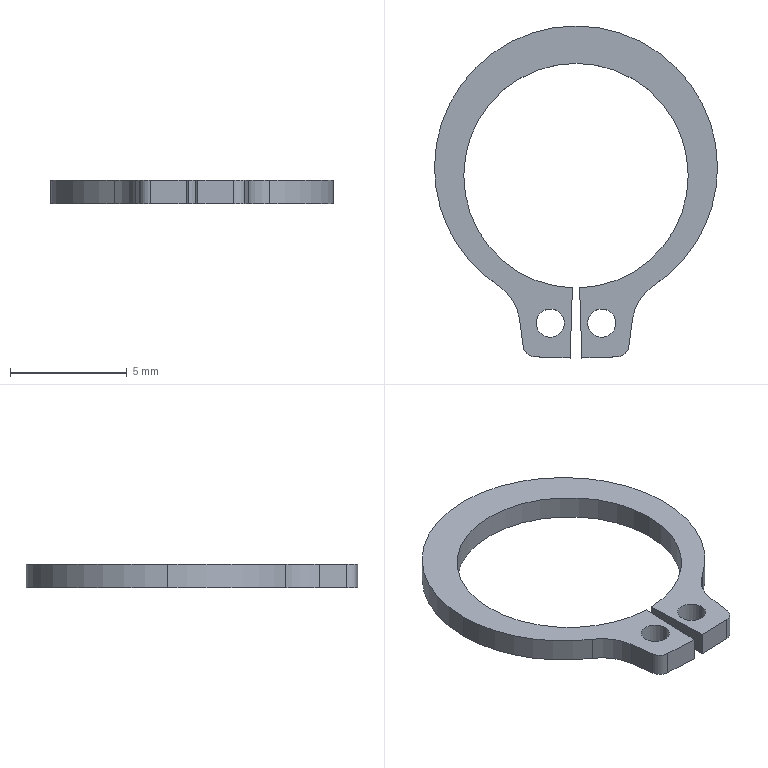Part | STEP file | C Type Shaft Use Retaining Ring_jis(PreviewCfg) | 1 solid | 22 faces | box 12.101 x 14.196 x 1 mm | volume 49.912 mm3 | cylinder 14 | plane 8 | commonest cylinder face diameters 1.2 x4 9.6 x3 12.101 x3 1 x2 4.078 x2